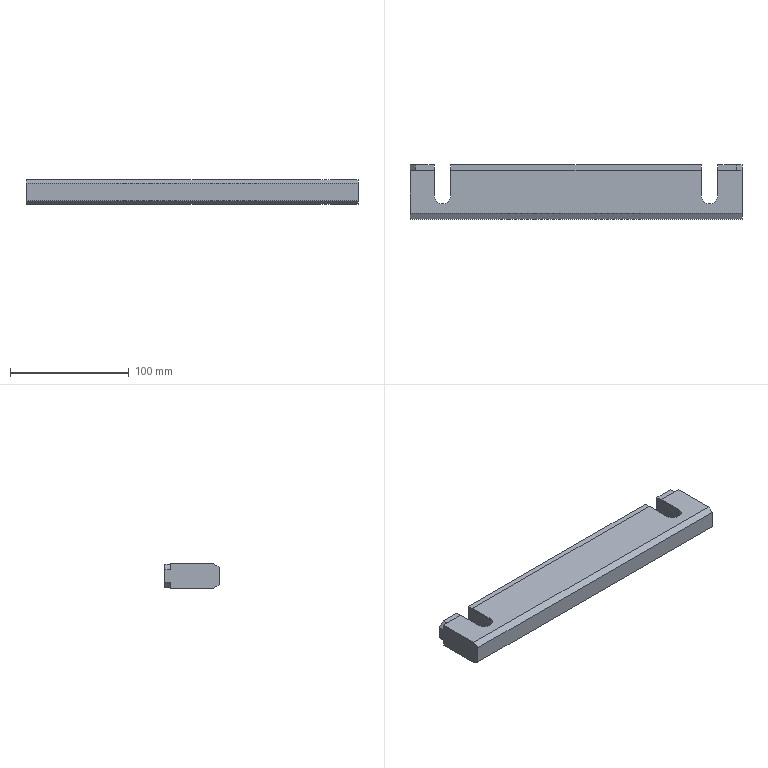Part | STEP file | 44-02-22 Ear Forming Locating Plate B | 1 solid | 40 faces | box 280 x 46 x 20.7 mm | volume 241213 mm3 | plane 30 | cylinder 6 | cone 4 | commonest cylinder face diameters 6.8 x4 14 x2